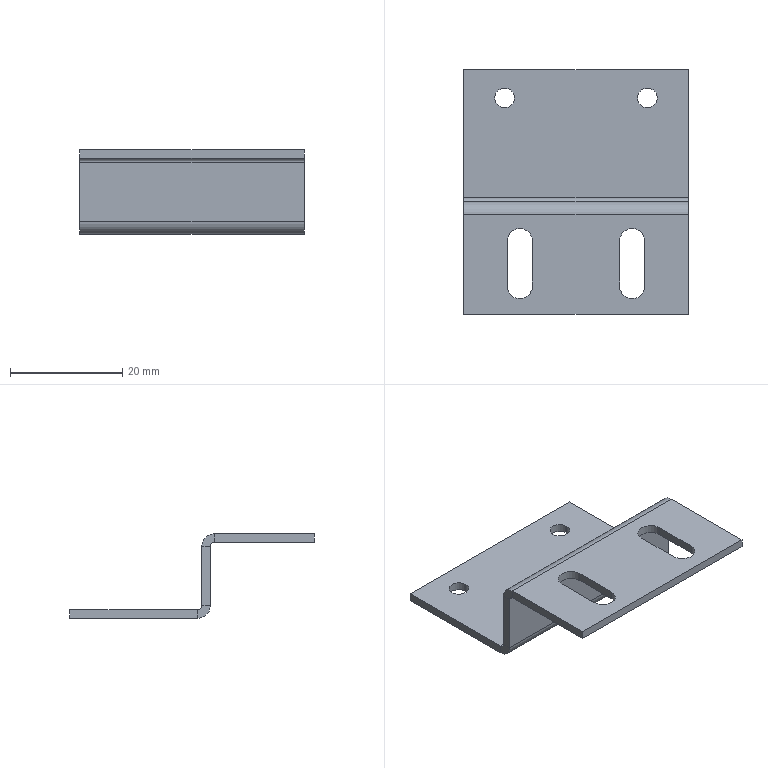Part | SolidWorks | features EdgeFlange 2, FlatPattern 1, ICE 1, SMBaseFlange 1, SheetMetal 1 | 1 solid | 34 faces | box 40 x 43.5 x 15 mm | volume 3159 mm3 | plane 22 | cylinder 12 | commonest cylinder face diameters 3.5 x4 4.5 x4 1.473 x2 4.473 x2
STEP:
#1=CARTESIAN_POINT('',(-14.45,28.5,-13.5));
#2=VERTEX_POINT('',#1);
#3=CARTESIAN_POINT('',(-10.95,28.5,-13.5));
#4=VERTEX_POINT('',#3);
#5=CARTESIAN_POINT('',(-12.7,28.5,-13.5));
#6=DIRECTION('',(0.,0.,1.));
#7=DIRECTION('',(1.,0.,0.));
#8=AXIS2_PLACEMENT_3D('',#5,#6,#7);
#9=CIRCLE('',#8,1.75);
#10=EDGE_CURVE('',#2,#4,#9,.T.);
#11=ORIENTED_EDGE('',*,*,#10,.T.);
#12=CARTESIAN_POINT('',(-10.95,28.5,-15.));
#13=VERTEX_POINT('',#12);
#14=CARTESIAN_POINT('',(-10.95,28.5,-5.));
#15=DIRECTION('',(0.,0.,-1.));
#16=VECTOR('',#15,1000.);
#17=LINE('',#14,#16);
#18=EDGE_CURVE('',#4,#13,#17,.T.);
#19=ORIENTED_EDGE('',*,*,#18,.T.);
#20=CARTESIAN_POINT('',(-14.45,28.5,-15.));
#21=VERTEX_POINT('',#20);
#22=CARTESIAN_POINT('',(-12.7,28.5,-15.));
#23=DIRECTION('',(0.,0.,-1.));
#24=DIRECTION('',(-1.,0.,0.));
#25=AXIS2_PLACEMENT_3D('',#22,#23,#24);
#26=CIRCLE('',#25,1.75);
#27=EDGE_CURVE('',#13,#21,#26,.T.);
#28=ORIENTED_EDGE('',*,*,#27,.T.);
#29=CARTESIAN_POINT('',(-14.45,28.5,-5.));
#30=DIRECTION('',(0.,0.,-1.));
#31=VECTOR('',#30,1000.);
#32=LINE('',#29,#31);
#33=EDGE_CURVE('',#2,#21,#32,.T.);
#34=ORIENTED_EDGE('',*,*,#33,.F.);
#35=EDGE_LOOP('',(#11,#19,#28,#34));
#36=FACE_OUTER_BOUND('',#35,.T.);
#37=CARTESIAN_POINT('',(-12.7,28.5,-5.));
#38=DIRECTION('',(0.,0.,-1.));
#39=DIRECTION('',(-1.,0.,0.));
#40=AXIS2_PLACEMENT_3D('',#37,#38,#39);
#41=CYLINDRICAL_SURFACE('',#40,1.75);
#42=ADVANCED_FACE('',(#36),#41,.F.);
#43=CARTESIAN_POINT('',(10.95,28.5,-13.5));
#44=VERTEX_POINT('',#43);
#45=CARTESIAN_POINT('',(14.45,28.5,-13.5));
#46=VERTEX_POINT('',#45);
#47=CARTESIAN_POINT('',(12.7,28.5,-13.5));
#48=DIRECTION('',(0.,0.,1.));
#49=DIRECTION('',(1.,0.,0.));
#50=AXIS2_PLACEMENT_3D('',#47,#48,#49);
#51=CIRCLE('',#50,1.75);
#52=EDGE_CURVE('',#44,#46,#51,.T.);
#53=ORIENTED_EDGE('',*,*,#52,.T.);
#54=CARTESIAN_POINT('',(14.45,28.5,-15.));
#55=VERTEX_POINT('',#54);
#56=CARTESIAN_POINT('',(14.45,28.5,-5.));
#57=DIRECTION('',(0.,0.,-1.));
#58=VECTOR('',#57,1000.);
#59=LINE('',#56,#58);
#60=EDGE_CURVE('',#46,#55,#59,.T.);
#61=ORIENTED_EDGE('',*,*,#60,.T.);
#62=CARTESIAN_POINT('',(10.95,28.5,-15.));
#63=VERTEX_POINT('',#62);
#64=CARTESIAN_POINT('',(12.7,28.5,-15.));
#65=DIRECTION('',(0.,0.,-1.));
#66=DIRECTION('',(-1.,0.,0.));
#67=AXIS2_PLACEMENT_3D('',#64,#65,#66);
#68=CIRCLE('',#67,1.75);
#69=EDGE_CURVE('',#55,#63,#68,.T.);
#70=ORIENTED_EDGE('',*,*,#69,.T.);
#71=CARTESIAN_POINT('',(10.95,28.5,-5.));
#72=DIRECTION('',(0.,0.,-1.));
#73=VECTOR('',#72,1000.);
#74=LINE('',#71,#73);
#75=EDGE_CURVE('',#44,#63,#74,.T.);
#76=ORIENTED_EDGE('',*,*,#75,.F.);
#77=EDGE_LOOP('',(#53,#61,#70,#76));
#78=FACE_OUTER_BOUND('',#77,.T.);
#79=CARTESIAN_POINT('',(12.7,28.5,-5.));
#80=DIRECTION('',(0.,0.,-1.));
#81=DIRECTION('',(-1.,0.,0.));
#82=AXIS2_PLACEMENT_3D('',#79,#80,#81);
#83=CYLINDRICAL_SURFACE('',#82,1.75);
#84=ADVANCED_FACE('',(#78),#83,.F.);
#85=CARTESIAN_POINT('',(-20.,10.,-2.237));
#86=VERTEX_POINT('',#85);
#87=CARTESIAN_POINT('',(-20.,10.,-12.763));
#88=VERTEX_POINT('',#87);
#89=CARTESIAN_POINT('',(-20.,10.,-15.));
#90=DIRECTION('',(0.,0.,-1.));
#91=VECTOR('',#90,1000.);
#92=LINE('',#89,#91);
#93=EDGE_CURVE('',#86,#88,#92,.T.);
#94=ORIENTED_EDGE('',*,*,#93,.T.);
#95=CARTESIAN_POINT('',(-20.,8.5,-12.763));
#96=VERTEX_POINT('',#95);
#97=CARTESIAN_POINT('',(-20.,10.,-12.763));
#98=DIRECTION('',(0.,-1.,0.));
#99=VECTOR('',#98,1000.);
#100=LINE('',#97,#99);
#101=EDGE_CURVE('',#88,#96,#100,.T.);
#102=ORIENTED_EDGE('',*,*,#101,.T.);
#103=CARTESIAN_POINT('',(-20.,8.5,-2.237));
#104=VERTEX_POINT('',#103);
#105=CARTESIAN_POINT('',(-20.,8.5,0.));
#106=DIRECTION('',(0.,0.,-1.));
#107=VECTOR('',#106,1000.);
#108=LINE('',#105,#107);
#109=EDGE_CURVE('',#104,#96,#108,.T.);
#110=ORIENTED_EDGE('',*,*,#109,.F.);
#111=CARTESIAN_POINT('',(-20.,10.,-2.237));
#112=DIRECTION('',(0.,1.,0.));
#113=VECTOR('',#112,1000.);
#114=LINE('',#111,#113);
#115=EDGE_CURVE('',#104,#86,#114,.T.);
#116=ORIENTED_EDGE('',*,*,#115,.T.);
#117=EDGE_LOOP('',(#94,#102,#110,#116));
#118=FACE_OUTER_BOUND('',#117,.T.);
#119=CARTESIAN_POINT('',(-20.,10.,-15.));
#120=DIRECTION('',(-1.,0.,0.));
#121=DIRECTION('',(0.,0.,1.));
#122=AXIS2_PLACEMENT_3D('',#119,#120,#121);
#123=PLANE('',#122);
#124=ADVANCED_FACE('',(#118),#123,.T.);
#125=CARTESIAN_POINT('',(20.,10.,-12.763));
#126=VERTEX_POINT('',#125);
#127=CARTESIAN_POINT('',(20.,10.,-2.237));
#128=VERTEX_POINT('',#127);
#129=CARTESIAN_POINT('',(20.,10.,-1.5));
#130=DIRECTION('',(0.,0.,1.));
#131=VECTOR('',#130,1000.);
#132=LINE('',#129,#131);
#133=EDGE_CURVE('',#126,#128,#132,.T.);
#134=ORIENTED_EDGE('',*,*,#133,.F.);
#135=CARTESIAN_POINT('',(-20.,10.,-12.763));
#136=DIRECTION('',(1.,0.,0.));
#137=VECTOR('',#136,1000.);
#138=LINE('',#135,#137);
#139=EDGE_CURVE('',#88,#126,#138,.T.);
#140=ORIENTED_EDGE('',*,*,#139,.F.);
#141=ORIENTED_EDGE('',*,*,#93,.F.);
#142=CARTESIAN_POINT('',(0.,10.,-2.237));
#143=DIRECTION('',(1.,0.,0.));
#144=VECTOR('',#143,1000.);
#145=LINE('',#142,#144);
#146=EDGE_CURVE('',#86,#128,#145,.T.);
#147=ORIENTED_EDGE('',*,*,#146,.T.);
#148=EDGE_LOOP('',(#134,#140,#141,#147));
#149=FACE_OUTER_BOUND('',#148,.T.);
#150=CARTESIAN_POINT('',(0.,10.,0.));
#151=DIRECTION('',(0.,1.,0.));
#152=DIRECTION('',(0.,0.,1.));
#153=AXIS2_PLACEMENT_3D('',#150,#151,#152);
#154=PLANE('',#153);
#155=ADVANCED_FACE('',(#149),#154,.T.);
#156=CARTESIAN_POINT('',(20.,8.5,-12.763));
#157=VERTEX_POINT('',#156);
#158=CARTESIAN_POINT('',(-20.,8.5,-12.763));
#159=DIRECTION('',(1.,0.,0.));
#160=VECTOR('',#159,1000.);
#161=LINE('',#158,#160);
#162=EDGE_CURVE('',#96,#157,#161,.T.);
#163=ORIENTED_EDGE('',*,*,#162,.T.);
#164=CARTESIAN_POINT('',(20.,8.5,-2.237));
#165=VERTEX_POINT('',#164);
#166=CARTESIAN_POINT('',(20.,8.5,0.));
#167=DIRECTION('',(0.,0.,1.));
#168=VECTOR('',#167,1000.);
#169=LINE('',#166,#168);
#170=EDGE_CURVE('',#157,#165,#169,.T.);
#171=ORIENTED_EDGE('',*,*,#170,.T.);
#172=CARTESIAN_POINT('',(-20.,8.5,-2.237));
#173=DIRECTION('',(1.,0.,0.));
#174=VECTOR('',#173,1000.);
#175=LINE('',#172,#174);
#176=EDGE_CURVE('',#104,#165,#175,.T.);
#177=ORIENTED_EDGE('',*,*,#176,.F.);
#178=ORIENTED_EDGE('',*,*,#109,.T.);
#179=EDGE_LOOP('',(#163,#171,#177,#178));
#180=FACE_OUTER_BOUND('',#179,.T.);
#181=CARTESIAN_POINT('',(0.,8.5,0.));
#182=DIRECTION('',(0.,1.,0.));
#183=DIRECTION('',(0.,0.,1.));
#184=AXIS2_PLACEMENT_3D('',#181,#182,#183);
#185=PLANE('',#184);
#186=ADVANCED_FACE('',(#180),#185,.F.);
#187=CARTESIAN_POINT('',(20.,-10.,-1.5));
#188=VERTEX_POINT('',#187);
#189=CARTESIAN_POINT('',(20.,7.763,-1.5));
#190=VERTEX_POINT('',#189);
#191=CARTESIAN_POINT('',(20.,10.,-1.5));
#192=DIRECTION('',(0.,1.,0.));
#193=VECTOR('',#192,1000.);
#194=LINE('',#191,#193);
#195=EDGE_CURVE('',#188,#190,#194,.T.);
#196=ORIENTED_EDGE('',*,*,#195,.T.);
#197=CARTESIAN_POINT('',(20.,7.763,0.));
#198=VERTEX_POINT('',#197);
#199=CARTESIAN_POINT('',(20.,7.763,-1.5));
#200=DIRECTION('',(0.,0.,1.));
#201=VECTOR('',#200,1000.);
#202=LINE('',#199,#201);
#203=EDGE_CURVE('',#190,#198,#202,.T.);
#204=ORIENTED_EDGE('',*,*,#203,.T.);
#205=CARTESIAN_POINT('',(20.,-10.,0.));
#206=VERTEX_POINT('',#205);
#207=CARTESIAN_POINT('',(20.,10.,0.));
#208=DIRECTION('',(0.,1.,0.));
#209=VECTOR('',#208,1000.);
#210=LINE('',#207,#209);
#211=EDGE_CURVE('',#206,#198,#210,.T.);
#212=ORIENTED_EDGE('',*,*,#211,.F.);
#213=CARTESIAN_POINT('',(20.,-10.,-1.5));
#214=DIRECTION('',(0.,0.,1.));
#215=VECTOR('',#214,1000.);
#216=LINE('',#213,#215);
#217=EDGE_CURVE('',#188,#206,#216,.T.);
#218=ORIENTED_EDGE('',*,*,#217,.F.);
#219=EDGE_LOOP('',(#196,#204,#212,#218));
#220=FACE_OUTER_BOUND('',#219,.T.);
#221=CARTESIAN_POINT('',(20.,10.,-1.5));
#222=DIRECTION('',(1.,0.,0.));
#223=DIRECTION('',(0.,0.,-1.));
#224=AXIS2_PLACEMENT_3D('',#221,#222,#223);
#225=PLANE('',#224);
#226=ADVANCED_FACE('',(#220),#225,.T.);
#227=CARTESIAN_POINT('',(-7.75,-5.,-1.5));
#228=VERTEX_POINT('',#227);
#229=CARTESIAN_POINT('',(-7.75,3.,-1.5));
#230=VERTEX_POINT('',#229);
#231=CARTESIAN_POINT('',(-7.75,3.,-1.5));
#232=DIRECTION('',(0.,1.,0.));
#233=VECTOR('',#232,1000.);
#234=LINE('',#231,#233);
#235=EDGE_CURVE('',#228,#230,#234,.T.);
#236=ORIENTED_EDGE('',*,*,#235,.T.);
#237=CARTESIAN_POINT('',(-12.25,3.,-1.5));
#238=VERTEX_POINT('',#237);
#239=CARTESIAN_POINT('',(-10.,3.,-1.5));
#240=DIRECTION('',(0.,0.,1.));
#241=DIRECTION('',(1.,0.,0.));
#242=AXIS2_PLACEMENT_3D('',#239,#240,#241);
#243=CIRCLE('',#242,2.25);
#244=EDGE_CURVE('',#230,#238,#243,.T.);
#245=ORIENTED_EDGE('',*,*,#244,.T.);
#246=CARTESIAN_POINT('',(-12.25,-5.,-1.5));
#247=VERTEX_POINT('',#246);
#248=CARTESIAN_POINT('',(-12.25,3.,-1.5));
#249=DIRECTION('',(0.,-1.,0.));
#250=VECTOR('',#249,1000.);
#251=LINE('',#248,#250);
#252=EDGE_CURVE('',#238,#247,#251,.T.);
#253=ORIENTED_EDGE('',*,*,#252,.T.);
#254=CARTESIAN_POINT('',(-10.,-5.,-1.5));
#255=DIRECTION('',(0.,0.,1.));
#256=DIRECTION('',(1.,0.,0.));
#257=AXIS2_PLACEMENT_3D('',#254,#255,#256);
#258=CIRCLE('',#257,2.25);
#259=EDGE_CURVE('',#247,#228,#258,.T.);
#260=ORIENTED_EDGE('',*,*,#259,.T.);
#261=EDGE_LOOP('',(#236,#245,#253,#260));
#262=FACE_BOUND('',#261,.T.);
#263=CARTESIAN_POINT('',(12.25,-5.,-1.5));
#264=VERTEX_POINT('',#263);
#265=CARTESIAN_POINT('',(12.25,3.,-1.5));
#266=VERTEX_POINT('',#265);
#267=CARTESIAN_POINT('',(12.25,3.,-1.5));
#268=DIRECTION('',(0.,1.,0.));
#269=VECTOR('',#268,1000.);
#270=LINE('',#267,#269);
#271=EDGE_CURVE('',#264,#266,#270,.T.);
#272=ORIENTED_EDGE('',*,*,#271,.T.);
#273=CARTESIAN_POINT('',(7.75,3.,-1.5));
#274=VERTEX_POINT('',#273);
#275=CARTESIAN_POINT('',(10.,3.,-1.5));
#276=DIRECTION('',(0.,0.,1.));
#277=DIRECTION('',(1.,0.,0.));
#278=AXIS2_PLACEMENT_3D('',#275,#276,#277);
#279=CIRCLE('',#278,2.25);
#280=EDGE_CURVE('',#266,#274,#279,.T.);
#281=ORIENTED_EDGE('',*,*,#280,.T.);
#282=CARTESIAN_POINT('',(7.75,-5.,-1.5));
#283=VERTEX_POINT('',#282);
#284=CARTESIAN_POINT('',(7.75,3.,-1.5));
#285=DIRECTION('',(0.,-1.,0.));
#286=VECTOR('',#285,1000.);
#287=LINE('',#284,#286);
#288=EDGE_CURVE('',#274,#283,#287,.T.);
#289=ORIENTED_EDGE('',*,*,#288,.T.);
#290=CARTESIAN_POINT('',(10.,-5.,-1.5));
#291=DIRECTION('',(0.,0.,1.));
#292=DIRECTION('',(1.,0.,0.));
#293=AXIS2_PLACEMENT_3D('',#290,#291,#292);
#294=CIRCLE('',#293,2.25);
#295=EDGE_CURVE('',#283,#264,#294,.T.);
#296=ORIENTED_EDGE('',*,*,#295,.T.);
#297=EDGE_LOOP('',(#272,#281,#289,#296));
#298=FACE_BOUND('',#297,.T.);
#299=CARTESIAN_POINT('',(-20.,7.763,-1.5));
#300=VERTEX_POINT('',#299);
#301=CARTESIAN_POINT('',(20.,7.763,-1.5));
#302=DIRECTION('',(-1.,0.,0.));
#303=VECTOR('',#302,1000.);
#304=LINE('',#301,#303);
#305=EDGE_CURVE('',#190,#300,#304,.T.);
#306=ORIENTED_EDGE('',*,*,#305,.F.);
#307=ORIENTED_EDGE('',*,*,#195,.F.);
#308=CARTESIAN_POINT('',(-20.,-10.,-1.5));
#309=VERTEX_POINT('',#308);
#310=CARTESIAN_POINT('',(-20.,-10.,-1.5));
#311=DIRECTION('',(1.,0.,0.));
#312=VECTOR('',#311,1000.);
#313=LINE('',#310,#312);
#314=EDGE_CURVE('',#309,#188,#313,.T.);
#315=ORIENTED_EDGE('',*,*,#314,.F.);
#316=CARTESIAN_POINT('',(-20.,10.,-1.5));
#317=DIRECTION('',(0.,-1.,0.));
#318=VECTOR('',#317,1000.);
#319=LINE('',#316,#318);
#320=EDGE_CURVE('',#300,#309,#319,.T.);
#321=ORIENTED_EDGE('',*,*,#320,.F.);
#322=EDGE_LOOP('',(#306,#307,#315,#321));
#323=FACE_OUTER_BOUND('',#322,.T.);
#324=CARTESIAN_POINT('',(0.,0.,-1.5));
#325=DIRECTION('',(0.,0.,1.));
#326=DIRECTION('',(1.,0.,0.));
#327=AXIS2_PLACEMENT_3D('',#324,#325,#326);
#328=PLANE('',#327);
#329=ADVANCED_FACE('',(#262,#298,#323),#328,.F.);
#330=CARTESIAN_POINT('',(-7.75,3.,0.));
#331=VERTEX_POINT('',#330);
#332=CARTESIAN_POINT('',(-12.25,3.,0.));
#333=VERTEX_POINT('',#332);
#334=CARTESIAN_POINT('',(-10.,3.,0.));
#335=DIRECTION('',(0.,0.,1.));
#336=DIRECTION('',(1.,0.,0.));
#337=AXIS2_PLACEMENT_3D('',#334,#335,#336);
#338=CIRCLE('',#337,2.25);
#339=EDGE_CURVE('',#331,#333,#338,.T.);
#340=ORIENTED_EDGE('',*,*,#339,.F.);
#341=CARTESIAN_POINT('',(-7.75,-5.,0.));
#342=VERTEX_POINT('',#341);
#343=CARTESIAN_POINT('',(-7.75,3.,0.));
#344=DIRECTION('',(0.,1.,0.));
#345=VECTOR('',#344,1000.);
#346=LINE('',#343,#345);
#347=EDGE_CURVE('',#342,#331,#346,.T.);
#348=ORIENTED_EDGE('',*,*,#347,.F.);
#349=CARTESIAN_POINT('',(-12.25,-5.,0.));
#350=VERTEX_POINT('',#349);
#351=CARTESIAN_POINT('',(-10.,-5.,0.));
#352=DIRECTION('',(0.,0.,1.));
#353=DIRECTION('',(1.,0.,0.));
#354=AXIS2_PLACEMENT_3D('',#351,#352,#353);
#355=CIRCLE('',#354,2.25);
#356=EDGE_CURVE('',#350,#342,#355,.T.);
#357=ORIENTED_EDGE('',*,*,#356,.F.);
#358=CARTESIAN_POINT('',(-12.25,3.,0.));
#359=DIRECTION('',(0.,-1.,0.));
#360=VECTOR('',#359,1000.);
#361=LINE('',#358,#360);
#362=EDGE_CURVE('',#333,#350,#361,.T.);
#363=ORIENTED_EDGE('',*,*,#362,.F.);
#364=EDGE_LOOP('',(#340,#348,#357,#363));
#365=FACE_BOUND('',#364,.T.);
#366=CARTESIAN_POINT('',(12.25,3.,0.));
#367=VERTEX_POINT('',#366);
#368=CARTESIAN_POINT('',(7.75,3.,0.));
#369=VERTEX_POINT('',#368);
#370=CARTESIAN_POINT('',(10.,3.,0.));
#371=DIRECTION('',(0.,0.,1.));
#372=DIRECTION('',(1.,0.,0.));
#373=AXIS2_PLACEMENT_3D('',#370,#371,#372);
#374=CIRCLE('',#373,2.25);
#375=EDGE_CURVE('',#367,#369,#374,.T.);
#376=ORIENTED_EDGE('',*,*,#375,.F.);
#377=CARTESIAN_POINT('',(12.25,-5.,0.));
#378=VERTEX_POINT('',#377);
#379=CARTESIAN_POINT('',(12.25,3.,0.));
#380=DIRECTION('',(0.,1.,0.));
#381=VECTOR('',#380,1000.);
#382=LINE('',#379,#381);
#383=EDGE_CURVE('',#378,#367,#382,.T.);
#384=ORIENTED_EDGE('',*,*,#383,.F.);
#385=CARTESIAN_POINT('',(7.75,-5.,0.));
#386=VERTEX_POINT('',#385);
#387=CARTESIAN_POINT('',(10.,-5.,0.));
#388=DIRECTION('',(0.,0.,1.));
#389=DIRECTION('',(1.,0.,0.));
#390=AXIS2_PLACEMENT_3D('',#387,#388,#389);
#391=CIRCLE('',#390,2.25);
#392=EDGE_CURVE('',#386,#378,#391,.T.);
#393=ORIENTED_EDGE('',*,*,#392,.F.);
#394=CARTESIAN_POINT('',(7.75,3.,0.));
#395=DIRECTION('',(0.,-1.,0.));
#396=VECTOR('',#395,1000.);
#397=LINE('',#394,#396);
#398=EDGE_CURVE('',#369,#386,#397,.T.);
#399=ORIENTED_EDGE('',*,*,#398,.F.);
#400=EDGE_LOOP('',(#376,#384,#393,#399));
#401=FACE_BOUND('',#400,.T.);
#402=ORIENTED_EDGE('',*,*,#211,.T.);
#403=CARTESIAN_POINT('',(-20.,7.763,0.));
#404=VERTEX_POINT('',#403);
#405=CARTESIAN_POINT('',(20.,7.763,0.));
#406=DIRECTION('',(-1.,0.,0.));
#407=VECTOR('',#406,1000.);
#408=LINE('',#405,#407);
#409=EDGE_CURVE('',#198,#404,#408,.T.);
#410=ORIENTED_EDGE('',*,*,#409,.T.);
#411=CARTESIAN_POINT('',(-20.,-10.,0.));
#412=VERTEX_POINT('',#411);
#413=CARTESIAN_POINT('',(-20.,10.,0.));
#414=DIRECTION('',(0.,-1.,0.));
#415=VECTOR('',#414,1000.);
#416=LINE('',#413,#415);
#417=EDGE_CURVE('',#404,#412,#416,.T.);
#418=ORIENTED_EDGE('',*,*,#417,.T.);
#419=CARTESIAN_POINT('',(-20.,-10.,0.));
#420=DIRECTION('',(1.,0.,0.));
#421=VECTOR('',#420,1000.);
#422=LINE('',#419,#421);
#423=EDGE_CURVE('',#412,#206,#422,.T.);
#424=ORIENTED_EDGE('',*,*,#423,.T.);
#425=EDGE_LOOP('',(#402,#410,#418,#424));
#426=FACE_OUTER_BOUND('',#425,.T.);
#427=CARTESIAN_POINT('',(0.,0.,0.));
#428=DIRECTION('',(0.,0.,1.));
#429=DIRECTION('',(1.,0.,0.));
#430=AXIS2_PLACEMENT_3D('',#427,#428,#429);
#431=PLANE('',#430);
#432=ADVANCED_FACE('',(#365,#401,#426),#431,.T.);
#433=ORIENTED_EDGE('',*,*,#423,.F.);
#434=CARTESIAN_POINT('',(-20.,-10.,-1.5));
#435=DIRECTION('',(0.,0.,1.));
#436=VECTOR('',#435,1000.);
#437=LINE('',#434,#436);
#438=EDGE_CURVE('',#309,#412,#437,.T.);
#439=ORIENTED_EDGE('',*,*,#438,.F.);
#440=ORIENTED_EDGE('',*,*,#314,.T.);
#441=ORIENTED_EDGE('',*,*,#217,.T.);
#442=EDGE_LOOP('',(#433,#439,#440,#441));
#443=FACE_OUTER_BOUND('',#442,.T.);
#444=CARTESIAN_POINT('',(-20.,-10.,-1.5));
#445=DIRECTION('',(0.,-1.,0.));
#446=DIRECTION('',(0.,0.,-1.));
#447=AXIS2_PLACEMENT_3D('',#444,#445,#446);
#448=PLANE('',#447);
#449=ADVANCED_FACE('',(#443),#448,.T.);
#450=CARTESIAN_POINT('',(-20.,7.763,-1.5));
#451=DIRECTION('',(0.,0.,1.));
#452=VECTOR('',#451,1000.);
#453=LINE('',#450,#452);
#454=EDGE_CURVE('',#300,#404,#453,.T.);
#455=ORIENTED_EDGE('',*,*,#454,.F.);
#456=ORIENTED_EDGE('',*,*,#320,.T.);
#457=ORIENTED_EDGE('',*,*,#438,.T.);
#458=ORIENTED_EDGE('',*,*,#417,.F.);
#459=EDGE_LOOP('',(#455,#456,#457,#458));
#460=FACE_OUTER_BOUND('',#459,.T.);
#461=CARTESIAN_POINT('',(-20.,10.,-1.5));
#462=DIRECTION('',(-1.,0.,0.));
#463=DIRECTION('',(0.,0.,1.));
#464=AXIS2_PLACEMENT_3D('',#461,#462,#463);
#465=PLANE('',#464);
#466=ADVANCED_FACE('',(#460),#465,.T.);
#467=ORIENTED_EDGE('',*,*,#339,.T.);
#468=CARTESIAN_POINT('',(-12.25,3.,-1.5));
#469=DIRECTION('',(0.,0.,1.));
#470=VECTOR('',#469,1000.);
#471=LINE('',#468,#470);
#472=EDGE_CURVE('',#238,#333,#471,.T.);
#473=ORIENTED_EDGE('',*,*,#472,.F.);
#474=ORIENTED_EDGE('',*,*,#244,.F.);
#475=CARTESIAN_POINT('',(-7.75,3.,-1.5));
#476=DIRECTION('',(0.,0.,1.));
#477=VECTOR('',#476,1000.);
#478=LINE('',#475,#477);
#479=EDGE_CURVE('',#230,#331,#478,.T.);
#480=ORIENTED_EDGE('',*,*,#479,.T.);
#481=EDGE_LOOP('',(#467,#473,#474,#480));
#482=FACE_OUTER_BOUND('',#481,.T.);
#483=CARTESIAN_POINT('',(-10.,3.,-1.5));
#484=DIRECTION('',(0.,0.,1.));
#485=DIRECTION('',(1.,0.,0.));
#486=AXIS2_PLACEMENT_3D('',#483,#484,#485);
#487=CYLINDRICAL_SURFACE('',#486,2.25);
#488=ADVANCED_FACE('',(#482),#487,.F.);
#489=ORIENTED_EDGE('',*,*,#347,.T.);
#490=ORIENTED_EDGE('',*,*,#479,.F.);
#491=ORIENTED_EDGE('',*,*,#235,.F.);
#492=CARTESIAN_POINT('',(-7.75,-5.,-1.5));
#493=DIRECTION('',(0.,0.,1.));
#494=VECTOR('',#493,1000.);
#495=LINE('',#492,#494);
#496=EDGE_CURVE('',#228,#342,#495,.T.);
#497=ORIENTED_EDGE('',*,*,#496,.T.);
#498=EDGE_LOOP('',(#489,#490,#491,#497));
#499=FACE_OUTER_BOUND('',#498,.T.);
#500=CARTESIAN_POINT('',(-7.75,3.,-1.5));
#501=DIRECTION('',(1.,0.,0.));
#502=DIRECTION('',(0.,0.,-1.));
#503=AXIS2_PLACEMENT_3D('',#500,#501,#502);
#504=PLANE('',#503);
#505=ADVANCED_FACE('',(#499),#504,.F.);
#506=ORIENTED_EDGE('',*,*,#356,.T.);
#507=ORIENTED_EDGE('',*,*,#496,.F.);
#508=ORIENTED_EDGE('',*,*,#259,.F.);
#509=CARTESIAN_POINT('',(-12.25,-5.,-1.5));
#510=DIRECTION('',(0.,0.,1.));
#511=VECTOR('',#510,1000.);
#512=LINE('',#509,#511);
#513=EDGE_CURVE('',#247,#350,#512,.T.);
#514=ORIENTED_EDGE('',*,*,#513,.T.);
#515=EDGE_LOOP('',(#506,#507,#508,#514));
#516=FACE_OUTER_BOUND('',#515,.T.);
#517=CARTESIAN_POINT('',(-10.,-5.,-1.5));
#518=DIRECTION('',(0.,0.,1.));
#519=DIRECTION('',(1.,0.,0.));
#520=AXIS2_PLACEMENT_3D('',#517,#518,#519);
#521=CYLINDRICAL_SURFACE('',#520,2.25);
#522=ADVANCED_FACE('',(#516),#521,.F.);
#523=ORIENTED_EDGE('',*,*,#362,.T.);
#524=ORIENTED_EDGE('',*,*,#513,.F.);
#525=ORIENTED_EDGE('',*,*,#252,.F.);
#526=ORIENTED_EDGE('',*,*,#472,.T.);
#527=EDGE_LOOP('',(#523,#524,#525,#526));
#528=FACE_OUTER_BOUND('',#527,.T.);
#529=CARTESIAN_POINT('',(-12.25,3.,-1.5));
#530=DIRECTION('',(-1.,0.,0.));
#531=DIRECTION('',(0.,-1.,0.));
#532=AXIS2_PLACEMENT_3D('',#529,#530,#531);
#533=PLANE('',#532);
#534=ADVANCED_FACE('',(#528),#533,.F.);
#535=ORIENTED_EDGE('',*,*,#375,.T.);
#536=CARTESIAN_POINT('',(7.75,3.,-1.5));
#537=DIRECTION('',(0.,0.,1.));
#538=VECTOR('',#537,1000.);
#539=LINE('',#536,#538);
#540=EDGE_CURVE('',#274,#369,#539,.T.);
#541=ORIENTED_EDGE('',*,*,#540,.F.);
#542=ORIENTED_EDGE('',*,*,#280,.F.);
#543=CARTESIAN_POINT('',(12.25,3.,-1.5));
#544=DIRECTION('',(0.,0.,1.));
#545=VECTOR('',#544,1000.);
#546=LINE('',#543,#545);
#547=EDGE_CURVE('',#266,#367,#546,.T.);
#548=ORIENTED_EDGE('',*,*,#547,.T.);
#549=EDGE_LOOP('',(#535,#541,#542,#548));
#550=FACE_OUTER_BOUND('',#549,.T.);
#551=CARTESIAN_POINT('',(10.,3.,-1.5));
#552=DIRECTION('',(0.,0.,1.));
#553=DIRECTION('',(1.,0.,0.));
#554=AXIS2_PLACEMENT_3D('',#551,#552,#553);
#555=CYLINDRICAL_SURFACE('',#554,2.25);
#556=ADVANCED_FACE('',(#550),#555,.F.);
#557=ORIENTED_EDGE('',*,*,#383,.T.);
#558=ORIENTED_EDGE('',*,*,#547,.F.);
#559=ORIENTED_EDGE('',*,*,#271,.F.);
#560=CARTESIAN_POINT('',(12.25,-5.,-1.5));
#561=DIRECTION('',(0.,0.,1.));
#562=VECTOR('',#561,1000.);
#563=LINE('',#560,#562);
#564=EDGE_CURVE('',#264,#378,#563,.T.);
#565=ORIENTED_EDGE('',*,*,#564,.T.);
#566=EDGE_LOOP('',(#557,#558,#559,#565));
#567=FACE_OUTER_BOUND('',#566,.T.);
#568=CARTESIAN_POINT('',(12.25,3.,-1.5));
#569=DIRECTION('',(1.,0.,0.));
#570=DIRECTION('',(0.,0.,-1.));
#571=AXIS2_PLACEMENT_3D('',#568,#569,#570);
#572=PLANE('',#571);
#573=ADVANCED_FACE('',(#567),#572,.F.);
#574=ORIENTED_EDGE('',*,*,#392,.T.);
#575=ORIENTED_EDGE('',*,*,#564,.F.);
#576=ORIENTED_EDGE('',*,*,#295,.F.);
#577=CARTESIAN_POINT('',(7.75,-5.,-1.5));
#578=DIRECTION('',(0.,0.,1.));
#579=VECTOR('',#578,1000.);
#580=LINE('',#577,#579);
#581=EDGE_CURVE('',#283,#386,#580,.T.);
#582=ORIENTED_EDGE('',*,*,#581,.T.);
#583=EDGE_LOOP('',(#574,#575,#576,#582));
#584=FACE_OUTER_BOUND('',#583,.T.);
#585=CARTESIAN_POINT('',(10.,-5.,-1.5));
#586=DIRECTION('',(0.,0.,1.));
#587=DIRECTION('',(1.,0.,0.));
#588=AXIS2_PLACEMENT_3D('',#585,#586,#587);
#589=CYLINDRICAL_SURFACE('',#588,2.25);
#590=ADVANCED_FACE('',(#584),#589,.F.);
#591=ORIENTED_EDGE('',*,*,#398,.T.);
#592=ORIENTED_EDGE('',*,*,#581,.F.);
#593=ORIENTED_EDGE('',*,*,#288,.F.);
#594=ORIENTED_EDGE('',*,*,#540,.T.);
#595=EDGE_LOOP('',(#591,#592,#593,#594));
#596=FACE_OUTER_BOUND('',#595,.T.);
#597=CARTESIAN_POINT('',(7.75,3.,-1.5));
#598=DIRECTION('',(-1.,0.,0.));
#599=DIRECTION('',(0.,-1.,0.));
#600=AXIS2_PLACEMENT_3D('',#597,#598,#599);
#601=PLANE('',#600);
#602=ADVANCED_FACE('',(#596),#601,.F.);
#603=ORIENTED_EDGE('',*,*,#115,.F.);
#604=CARTESIAN_POINT('',(-20.,7.763,-2.237));
#605=DIRECTION('',(-1.,0.,0.));
#606=DIRECTION('',(0.,0.,-1.));
#607=AXIS2_PLACEMENT_3D('',#604,#605,#606);
#608=CIRCLE('',#607,0.7366);
#609=EDGE_CURVE('',#300,#104,#608,.T.);
#610=ORIENTED_EDGE('',*,*,#609,.F.);
#611=ORIENTED_EDGE('',*,*,#454,.T.);
#612=CARTESIAN_POINT('',(-20.,7.763,-2.237));
#613=DIRECTION('',(-1.,0.,0.));
#614=DIRECTION('',(0.,0.,-1.));
#615=AXIS2_PLACEMENT_3D('',#612,#613,#614);
#616=CIRCLE('',#615,2.237);
#617=EDGE_CURVE('',#404,#86,#616,.T.);
#618=ORIENTED_EDGE('',*,*,#617,.T.);
#619=EDGE_LOOP('',(#603,#610,#611,#618));
#620=FACE_OUTER_BOUND('',#619,.T.);
#621=CARTESIAN_POINT('',(-20.,7.763,-2.237));
#622=DIRECTION('',(-1.,0.,0.));
#623=DIRECTION('',(0.,0.,1.));
#624=AXIS2_PLACEMENT_3D('',#621,#622,#623);
#625=PLANE('',#624);
#626=ADVANCED_FACE('',(#620),#625,.T.);
#627=CARTESIAN_POINT('',(20.,7.763,-2.237));
#628=DIRECTION('',(1.,0.,0.));
#629=DIRECTION('',(0.,0.,-1.));
#630=AXIS2_PLACEMENT_3D('',#627,#628,#629);
#631=CIRCLE('',#630,0.7366);
#632=EDGE_CURVE('',#165,#190,#631,.T.);
#633=ORIENTED_EDGE('',*,*,#632,.F.);
#634=CARTESIAN_POINT('',(20.,8.5,-2.237));
#635=DIRECTION('',(0.,1.,0.));
#636=VECTOR('',#635,1000.);
#637=LINE('',#634,#636);
#638=EDGE_CURVE('',#165,#128,#637,.T.);
#639=ORIENTED_EDGE('',*,*,#638,.T.);
#640=CARTESIAN_POINT('',(20.,7.763,-2.237));
#641=DIRECTION('',(1.,0.,0.));
#642=DIRECTION('',(0.,0.,-1.));
#643=AXIS2_PLACEMENT_3D('',#640,#641,#642);
#644=CIRCLE('',#643,2.237);
#645=EDGE_CURVE('',#128,#198,#644,.T.);
#646=ORIENTED_EDGE('',*,*,#645,.T.);
#647=ORIENTED_EDGE('',*,*,#203,.F.);
#648=EDGE_LOOP('',(#633,#639,#646,#647));
#649=FACE_OUTER_BOUND('',#648,.T.);
#650=CARTESIAN_POINT('',(20.,7.763,-2.237));
#651=DIRECTION('',(-1.,0.,0.));
#652=DIRECTION('',(0.,0.,1.));
#653=AXIS2_PLACEMENT_3D('',#650,#651,#652);
#654=PLANE('',#653);
#655=ADVANCED_FACE('',(#649),#654,.F.);
#656=ORIENTED_EDGE('',*,*,#409,.F.);
#657=ORIENTED_EDGE('',*,*,#645,.F.);
#658=ORIENTED_EDGE('',*,*,#146,.F.);
#659=ORIENTED_EDGE('',*,*,#617,.F.);
#660=EDGE_LOOP('',(#656,#657,#658,#659));
#661=FACE_OUTER_BOUND('',#660,.T.);
#662=CARTESIAN_POINT('',(20.,7.763,-2.237));
#663=DIRECTION('',(1.,0.,0.));
#664=DIRECTION('',(0.,1.,0.));
#665=AXIS2_PLACEMENT_3D('',#662,#663,#664);
#666=CYLINDRICAL_SURFACE('',#665,2.237);
#667=ADVANCED_FACE('',(#661),#666,.T.);
#668=ORIENTED_EDGE('',*,*,#305,.T.);
#669=ORIENTED_EDGE('',*,*,#609,.T.);
#670=ORIENTED_EDGE('',*,*,#176,.T.);
#671=ORIENTED_EDGE('',*,*,#632,.T.);
#672=EDGE_LOOP('',(#668,#669,#670,#671));
#673=FACE_OUTER_BOUND('',#672,.T.);
#674=CARTESIAN_POINT('',(20.,7.763,-2.237));
#675=DIRECTION('',(1.,0.,0.));
#676=DIRECTION('',(0.,1.,0.));
#677=AXIS2_PLACEMENT_3D('',#674,#675,#676);
#678=CYLINDRICAL_SURFACE('',#677,0.7366);
#679=ADVANCED_FACE('',(#673),#678,.F.);
#680=CARTESIAN_POINT('',(20.,10.,-12.763));
#681=DIRECTION('',(0.,-1.,0.));
#682=VECTOR('',#681,1000.);
#683=LINE('',#680,#682);
#684=EDGE_CURVE('',#126,#157,#683,.T.);
#685=ORIENTED_EDGE('',*,*,#684,.F.);
#686=ORIENTED_EDGE('',*,*,#133,.T.);
#687=ORIENTED_EDGE('',*,*,#638,.F.);
#688=ORIENTED_EDGE('',*,*,#170,.F.);
#689=EDGE_LOOP('',(#685,#686,#687,#688));
#690=FACE_OUTER_BOUND('',#689,.T.);
#691=CARTESIAN_POINT('',(20.,10.,-1.5));
#692=DIRECTION('',(1.,0.,0.));
#693=DIRECTION('',(0.,0.,-1.));
#694=AXIS2_PLACEMENT_3D('',#691,#692,#693);
#695=PLANE('',#694);
#696=ADVANCED_FACE('',(#690),#695,.T.);
#697=CARTESIAN_POINT('',(20.,10.737,-13.5));
#698=VERTEX_POINT('',#697);
#699=CARTESIAN_POINT('',(20.,10.737,-15.));
#700=VERTEX_POINT('',#699);
#701=CARTESIAN_POINT('',(20.,10.737,-15.));
#702=DIRECTION('',(0.,0.,-1.));
#703=VECTOR('',#702,1000.);
#704=LINE('',#701,#703);
#705=EDGE_CURVE('',#698,#700,#704,.T.);
#706=ORIENTED_EDGE('',*,*,#705,.F.);
#707=CARTESIAN_POINT('',(20.,10.737,-12.763));
#708=DIRECTION('',(1.,0.,0.));
#709=DIRECTION('',(0.,0.,1.));
#710=AXIS2_PLACEMENT_3D('',#707,#708,#709);
#711=CIRCLE('',#710,0.7366);
#712=EDGE_CURVE('',#126,#698,#711,.T.);
#713=ORIENTED_EDGE('',*,*,#712,.F.);
#714=ORIENTED_EDGE('',*,*,#684,.T.);
#715=CARTESIAN_POINT('',(20.,10.737,-12.763));
#716=DIRECTION('',(1.,0.,0.));
#717=DIRECTION('',(0.,0.,1.));
#718=AXIS2_PLACEMENT_3D('',#715,#716,#717);
#719=CIRCLE('',#718,2.237);
#720=EDGE_CURVE('',#157,#700,#719,.T.);
#721=ORIENTED_EDGE('',*,*,#720,.T.);
#722=EDGE_LOOP('',(#706,#713,#714,#721));
#723=FACE_OUTER_BOUND('',#722,.T.);
#724=CARTESIAN_POINT('',(20.,10.737,-12.763));
#725=DIRECTION('',(1.,0.,0.));
#726=DIRECTION('',(0.,0.,-1.));
#727=AXIS2_PLACEMENT_3D('',#724,#725,#726);
#728=PLANE('',#727);
#729=ADVANCED_FACE('',(#723),#728,.T.);
#730=CARTESIAN_POINT('',(-20.,10.737,-13.5));
#731=VERTEX_POINT('',#730);
#732=CARTESIAN_POINT('',(-20.,10.737,-12.763));
#733=DIRECTION('',(-1.,0.,0.));
#734=DIRECTION('',(0.,0.,1.));
#735=AXIS2_PLACEMENT_3D('',#732,#733,#734);
#736=CIRCLE('',#735,0.7366);
#737=EDGE_CURVE('',#731,#88,#736,.T.);
#738=ORIENTED_EDGE('',*,*,#737,.F.);
#739=CARTESIAN_POINT('',(-20.,10.737,-15.));
#740=VERTEX_POINT('',#739);
#741=CARTESIAN_POINT('',(-20.,10.737,-13.5));
#742=DIRECTION('',(0.,0.,-1.));
#743=VECTOR('',#742,1000.);
#744=LINE('',#741,#743);
#745=EDGE_CURVE('',#731,#740,#744,.T.);
#746=ORIENTED_EDGE('',*,*,#745,.T.);
#747=CARTESIAN_POINT('',(-20.,10.737,-12.763));
#748=DIRECTION('',(-1.,0.,0.));
#749=DIRECTION('',(0.,0.,1.));
#750=AXIS2_PLACEMENT_3D('',#747,#748,#749);
#751=CIRCLE('',#750,2.237);
#752=EDGE_CURVE('',#740,#96,#751,.T.);
#753=ORIENTED_EDGE('',*,*,#752,.T.);
#754=ORIENTED_EDGE('',*,*,#101,.F.);
#755=EDGE_LOOP('',(#738,#746,#753,#754));
#756=FACE_OUTER_BOUND('',#755,.T.);
#757=CARTESIAN_POINT('',(-20.,10.737,-12.763));
#758=DIRECTION('',(1.,0.,0.));
#759=DIRECTION('',(0.,0.,-1.));
#760=AXIS2_PLACEMENT_3D('',#757,#758,#759);
#761=PLANE('',#760);
#762=ADVANCED_FACE('',(#756),#761,.F.);
#763=ORIENTED_EDGE('',*,*,#162,.F.);
#764=ORIENTED_EDGE('',*,*,#752,.F.);
#765=CARTESIAN_POINT('',(20.,10.737,-15.));
#766=DIRECTION('',(1.,0.,0.));
#767=VECTOR('',#766,1000.);
#768=LINE('',#765,#767);
#769=EDGE_CURVE('',#740,#700,#768,.T.);
#770=ORIENTED_EDGE('',*,*,#769,.T.);
#771=ORIENTED_EDGE('',*,*,#720,.F.);
#772=EDGE_LOOP('',(#763,#764,#770,#771));
#773=FACE_OUTER_BOUND('',#772,.T.);
#774=CARTESIAN_POINT('',(-20.,10.737,-12.763));
#775=DIRECTION('',(-1.,0.,0.));
#776=DIRECTION('',(0.,0.,-1.));
#777=AXIS2_PLACEMENT_3D('',#774,#775,#776);
#778=CYLINDRICAL_SURFACE('',#777,2.237);
#779=ADVANCED_FACE('',(#773),#778,.T.);
#780=ORIENTED_EDGE('',*,*,#139,.T.);
#781=ORIENTED_EDGE('',*,*,#712,.T.);
#782=CARTESIAN_POINT('',(20.,10.737,-13.5));
#783=DIRECTION('',(-1.,0.,0.));
#784=VECTOR('',#783,1000.);
#785=LINE('',#782,#784);
#786=EDGE_CURVE('',#698,#731,#785,.T.);
#787=ORIENTED_EDGE('',*,*,#786,.T.);
#788=ORIENTED_EDGE('',*,*,#737,.T.);
#789=EDGE_LOOP('',(#780,#781,#787,#788));
#790=FACE_OUTER_BOUND('',#789,.T.);
#791=CARTESIAN_POINT('',(-20.,10.737,-12.763));
#792=DIRECTION('',(-1.,0.,0.));
#793=DIRECTION('',(0.,0.,-1.));
#794=AXIS2_PLACEMENT_3D('',#791,#792,#793);
#795=CYLINDRICAL_SURFACE('',#794,0.7366);
#796=ADVANCED_FACE('',(#790),#795,.F.);
#797=ORIENTED_EDGE('',*,*,#745,.F.);
#798=CARTESIAN_POINT('',(-20.,33.5,-13.5));
#799=VERTEX_POINT('',#798);
#800=CARTESIAN_POINT('',(-20.,33.5,-13.5));
#801=DIRECTION('',(0.,1.,0.));
#802=VECTOR('',#801,1000.);
#803=LINE('',#800,#802);
#804=EDGE_CURVE('',#731,#799,#803,.T.);
#805=ORIENTED_EDGE('',*,*,#804,.T.);
#806=CARTESIAN_POINT('',(-20.,33.5,-15.));
#807=VERTEX_POINT('',#806);
#808=CARTESIAN_POINT('',(-20.,33.5,-15.));
#809=DIRECTION('',(0.,0.,1.));
#810=VECTOR('',#809,1000.);
#811=LINE('',#808,#810);
#812=EDGE_CURVE('',#807,#799,#811,.T.);
#813=ORIENTED_EDGE('',*,*,#812,.F.);
#814=CARTESIAN_POINT('',(-20.,0.,-15.));
#815=DIRECTION('',(0.,1.,0.));
#816=VECTOR('',#815,1000.);
#817=LINE('',#814,#816);
#818=EDGE_CURVE('',#740,#807,#817,.T.);
#819=ORIENTED_EDGE('',*,*,#818,.F.);
#820=EDGE_LOOP('',(#797,#805,#813,#819));
#821=FACE_OUTER_BOUND('',#820,.T.);
#822=CARTESIAN_POINT('',(-20.,33.5,-15.));
#823=DIRECTION('',(1.,0.,0.));
#824=DIRECTION('',(0.,0.,-1.));
#825=AXIS2_PLACEMENT_3D('',#822,#823,#824);
#826=PLANE('',#825);
#827=ADVANCED_FACE('',(#821),#826,.F.);
#828=ORIENTED_EDGE('',*,*,#705,.T.);
#829=CARTESIAN_POINT('',(20.,33.5,-15.));
#830=VERTEX_POINT('',#829);
#831=CARTESIAN_POINT('',(20.,0.,-15.));
#832=DIRECTION('',(0.,-1.,0.));
#833=VECTOR('',#832,1000.);
#834=LINE('',#831,#833);
#835=EDGE_CURVE('',#830,#700,#834,.T.);
#836=ORIENTED_EDGE('',*,*,#835,.F.);
#837=CARTESIAN_POINT('',(20.,33.5,-13.5));
#838=VERTEX_POINT('',#837);
#839=CARTESIAN_POINT('',(20.,33.5,-15.));
#840=DIRECTION('',(0.,0.,1.));
#841=VECTOR('',#840,1000.);
#842=LINE('',#839,#841);
#843=EDGE_CURVE('',#830,#838,#842,.T.);
#844=ORIENTED_EDGE('',*,*,#843,.T.);
#845=CARTESIAN_POINT('',(20.,10.,-13.5));
#846=DIRECTION('',(0.,-1.,0.));
#847=VECTOR('',#846,1000.);
#848=LINE('',#845,#847);
#849=EDGE_CURVE('',#838,#698,#848,.T.);
#850=ORIENTED_EDGE('',*,*,#849,.T.);
#851=EDGE_LOOP('',(#828,#836,#844,#850));
#852=FACE_OUTER_BOUND('',#851,.T.);
#853=CARTESIAN_POINT('',(20.,10.,-15.));
#854=DIRECTION('',(-1.,0.,0.));
#855=DIRECTION('',(0.,0.,1.));
#856=AXIS2_PLACEMENT_3D('',#853,#854,#855);
#857=PLANE('',#856);
#858=ADVANCED_FACE('',(#852),#857,.F.);
#859=CARTESIAN_POINT('',(-12.7,28.5,-15.));
#860=DIRECTION('',(0.,0.,-1.));
#861=DIRECTION('',(-1.,0.,0.));
#862=AXIS2_PLACEMENT_3D('',#859,#860,#861);
#863=CIRCLE('',#862,1.75);
#864=EDGE_CURVE('',#21,#13,#863,.T.);
#865=ORIENTED_EDGE('',*,*,#864,.F.);
#866=ORIENTED_EDGE('',*,*,#27,.F.);
#867=EDGE_LOOP('',(#865,#866));
#868=FACE_BOUND('',#867,.T.);
#869=CARTESIAN_POINT('',(12.7,28.5,-15.));
#870=DIRECTION('',(0.,0.,-1.));
#871=DIRECTION('',(-1.,0.,0.));
#872=AXIS2_PLACEMENT_3D('',#869,#870,#871);
#873=CIRCLE('',#872,1.75);
#874=EDGE_CURVE('',#63,#55,#873,.T.);
#875=ORIENTED_EDGE('',*,*,#874,.F.);
#876=ORIENTED_EDGE('',*,*,#69,.F.);
#877=EDGE_LOOP('',(#875,#876));
#878=FACE_BOUND('',#877,.T.);
#879=ORIENTED_EDGE('',*,*,#769,.F.);
#880=ORIENTED_EDGE('',*,*,#818,.T.);
#881=CARTESIAN_POINT('',(0.,33.5,-15.));
#882=DIRECTION('',(1.,0.,0.));
#883=VECTOR('',#882,1000.);
#884=LINE('',#881,#883);
#885=EDGE_CURVE('',#807,#830,#884,.T.);
#886=ORIENTED_EDGE('',*,*,#885,.T.);
#887=ORIENTED_EDGE('',*,*,#835,.T.);
#888=EDGE_LOOP('',(#879,#880,#886,#887));
#889=FACE_OUTER_BOUND('',#888,.T.);
#890=CARTESIAN_POINT('',(0.,0.,-15.));
#891=DIRECTION('',(0.,0.,1.));
#892=DIRECTION('',(1.,0.,0.));
#893=AXIS2_PLACEMENT_3D('',#890,#891,#892);
#894=PLANE('',#893);
#895=ADVANCED_FACE('',(#868,#878,#889),#894,.F.);
#896=ORIENTED_EDGE('',*,*,#10,.F.);
#897=CARTESIAN_POINT('',(-12.7,28.5,-13.5));
#898=DIRECTION('',(0.,0.,1.));
#899=DIRECTION('',(1.,0.,0.));
#900=AXIS2_PLACEMENT_3D('',#897,#898,#899);
#901=CIRCLE('',#900,1.75);
#902=EDGE_CURVE('',#4,#2,#901,.T.);
#903=ORIENTED_EDGE('',*,*,#902,.F.);
#904=EDGE_LOOP('',(#896,#903));
#905=FACE_BOUND('',#904,.T.);
#906=ORIENTED_EDGE('',*,*,#52,.F.);
#907=CARTESIAN_POINT('',(12.7,28.5,-13.5));
#908=DIRECTION('',(0.,0.,1.));
#909=DIRECTION('',(1.,0.,0.));
#910=AXIS2_PLACEMENT_3D('',#907,#908,#909);
#911=CIRCLE('',#910,1.75);
#912=EDGE_CURVE('',#46,#44,#911,.T.);
#913=ORIENTED_EDGE('',*,*,#912,.F.);
#914=EDGE_LOOP('',(#906,#913));
#915=FACE_BOUND('',#914,.T.);
#916=ORIENTED_EDGE('',*,*,#804,.F.);
#917=ORIENTED_EDGE('',*,*,#786,.F.);
#918=ORIENTED_EDGE('',*,*,#849,.F.);
#919=CARTESIAN_POINT('',(20.,33.5,-13.5));
#920=DIRECTION('',(1.,0.,0.));
#921=VECTOR('',#920,1000.);
#922=LINE('',#919,#921);
#923=EDGE_CURVE('',#799,#838,#922,.T.);
#924=ORIENTED_EDGE('',*,*,#923,.F.);
#925=EDGE_LOOP('',(#916,#917,#918,#924));
#926=FACE_OUTER_BOUND('',#925,.T.);
#927=CARTESIAN_POINT('',(0.,0.,-13.5));
#928=DIRECTION('',(0.,0.,1.));
#929=DIRECTION('',(1.,0.,0.));
#930=AXIS2_PLACEMENT_3D('',#927,#928,#929);
#931=PLANE('',#930);
#932=ADVANCED_FACE('',(#905,#915,#926),#931,.T.);
#933=ORIENTED_EDGE('',*,*,#923,.T.);
#934=ORIENTED_EDGE('',*,*,#843,.F.);
#935=ORIENTED_EDGE('',*,*,#885,.F.);
#936=ORIENTED_EDGE('',*,*,#812,.T.);
#937=EDGE_LOOP('',(#933,#934,#935,#936));
#938=FACE_OUTER_BOUND('',#937,.T.);
#939=CARTESIAN_POINT('',(20.,33.5,-15.));
#940=DIRECTION('',(0.,-1.,0.));
#941=DIRECTION('',(0.,0.,-1.));
#942=AXIS2_PLACEMENT_3D('',#939,#940,#941);
#943=PLANE('',#942);
#944=ADVANCED_FACE('',(#938),#943,.F.);
#945=ORIENTED_EDGE('',*,*,#60,.F.);
#946=ORIENTED_EDGE('',*,*,#912,.T.);
#947=ORIENTED_EDGE('',*,*,#75,.T.);
#948=ORIENTED_EDGE('',*,*,#874,.T.);
#949=EDGE_LOOP('',(#945,#946,#947,#948));
#950=FACE_OUTER_BOUND('',#949,.T.);
#951=CARTESIAN_POINT('',(12.7,28.5,-5.));
#952=DIRECTION('',(0.,0.,-1.));
#953=DIRECTION('',(-1.,0.,0.));
#954=AXIS2_PLACEMENT_3D('',#951,#952,#953);
#955=CYLINDRICAL_SURFACE('',#954,1.75);
#956=ADVANCED_FACE('',(#950),#955,.F.);
#957=ORIENTED_EDGE('',*,*,#18,.F.);
#958=ORIENTED_EDGE('',*,*,#902,.T.);
#959=ORIENTED_EDGE('',*,*,#33,.T.);
#960=ORIENTED_EDGE('',*,*,#864,.T.);
#961=EDGE_LOOP('',(#957,#958,#959,#960));
#962=FACE_OUTER_BOUND('',#961,.T.);
#963=CARTESIAN_POINT('',(-12.7,28.5,-5.));
#964=DIRECTION('',(0.,0.,-1.));
#965=DIRECTION('',(-1.,0.,0.));
#966=AXIS2_PLACEMENT_3D('',#963,#964,#965);
#967=CYLINDRICAL_SURFACE('',#966,1.75);
#968=ADVANCED_FACE('',(#962),#967,.F.);
#969=CLOSED_SHELL('',(#42,#84,#124,#155,#186,#226,#329,#432,#449,#466,#488,#505,#522,#534,#556,#573,#590,#602,#626,#655,#667,#679,#696,#729,#762,#779,#796,#827,#858,#895,#932,#944,#956,#968));
#970=MANIFOLD_SOLID_BREP('',#969);
#971=CARTESIAN_POINT('',(0.,0.,0.));
#972=DIRECTION('',(0.,0.,1.));
#973=DIRECTION('',(1.,0.,0.));
#974=AXIS2_PLACEMENT_3D('',#971,#972,#973);
#975=(LENGTH_UNIT()NAMED_UNIT(*)SI_UNIT(.MILLI.,.METRE.));
#976=UNCERTAINTY_MEASURE_WITH_UNIT(LENGTH_MEASURE(0.00001),#975,'','');
#977=(NAMED_UNIT(*)PLANE_ANGLE_UNIT()SI_UNIT($,.RADIAN.));
#978=(NAMED_UNIT(*)SI_UNIT($,.STERADIAN.)SOLID_ANGLE_UNIT());
#979=(GEOMETRIC_REPRESENTATION_CONTEXT(3)GLOBAL_UNCERTAINTY_ASSIGNED_CONTEXT((#976))GLOBAL_UNIT_ASSIGNED_CONTEXT((#975,#977,#978))REPRESENTATION_CONTEXT('',''));
#980=ADVANCED_BREP_SHAPE_REPRESENTATION('',(#970,#974),#979);